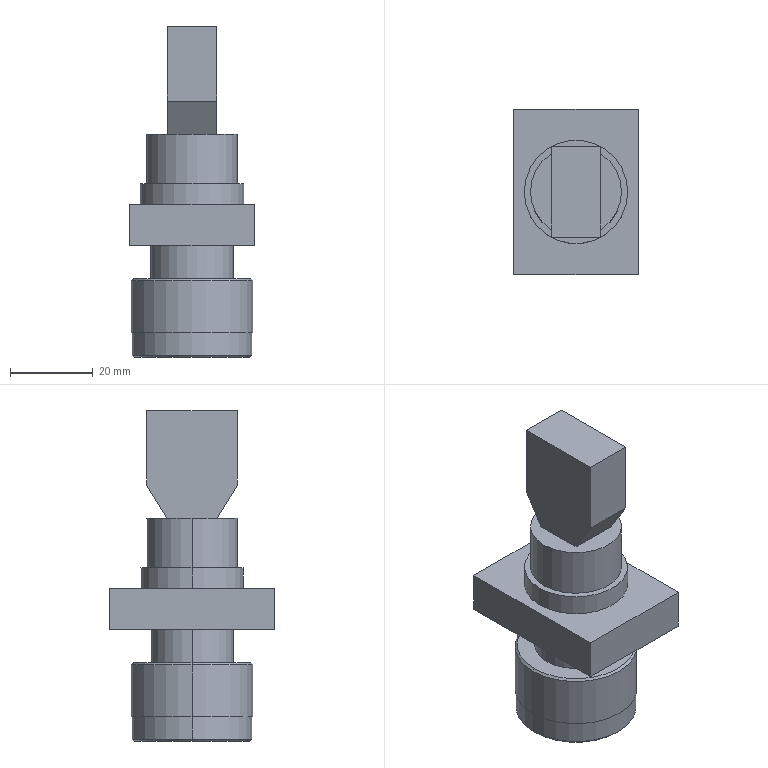Part | STEP file | Green illuminated pushbutton XB2-BW33B1C with 1 NO contact | 1 solid | 32 faces | box 30 x 40 x 80 mm | volume 40739 mm3 | plane 18 | cylinder 10 | cone 4 | commonest cylinder face diameters 20 x2 22 x2 25 x2 29 x2 29.5 x2